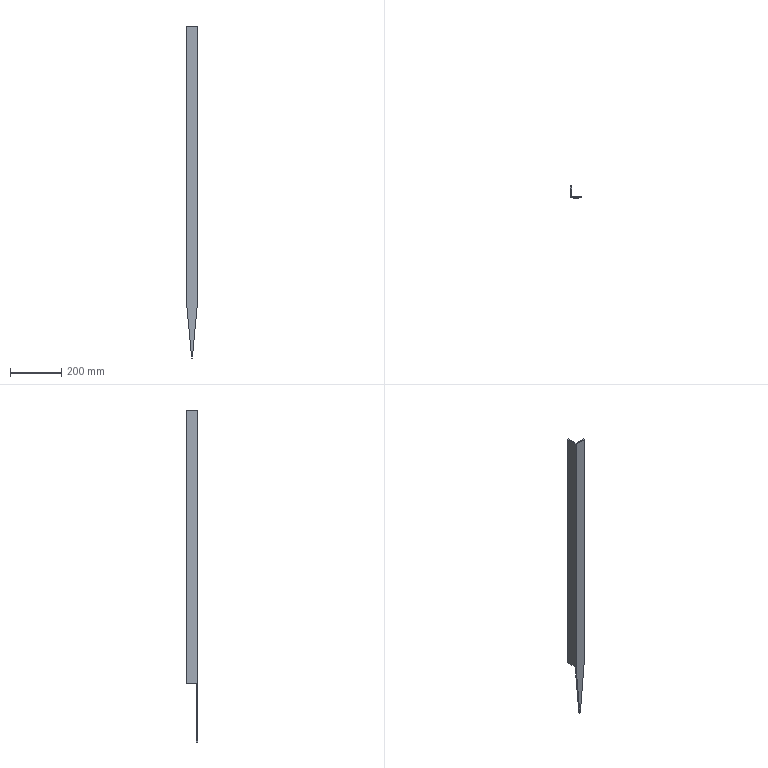Part | SolidWorks | features ICE 2, Extrusion 1 | 1 solid | 11 faces | box 45 x 45 x 1295 mm | volume 480925 mm3 | plane 11
STEP:
#1=CARTESIAN_POINT('',(-6.005,1.14,1295.4));
#2=VERTEX_POINT('',#1);
#3=CARTESIAN_POINT('',(-6.005,1.14,228.6));
#4=VERTEX_POINT('',#3);
#5=CARTESIAN_POINT('',(-6.005,1.14,1295.4));
#6=DIRECTION('',(0.,0.,-1.));
#7=VECTOR('',#6,1000.);
#8=LINE('',#5,#7);
#9=EDGE_CURVE('',#2,#4,#8,.T.);
#10=ORIENTED_EDGE('',*,*,#9,.T.);
#11=CARTESIAN_POINT('',(-11.005,1.14,228.6));
#12=VERTEX_POINT('',#11);
#13=CARTESIAN_POINT('',(-11.005,1.14,228.6));
#14=DIRECTION('',(1.,0.,0.));
#15=VECTOR('',#14,1000.);
#16=LINE('',#13,#15);
#17=EDGE_CURVE('',#12,#4,#16,.T.);
#18=ORIENTED_EDGE('',*,*,#17,.F.);
#19=CARTESIAN_POINT('',(-11.005,1.14,1295.4));
#20=VERTEX_POINT('',#19);
#21=CARTESIAN_POINT('',(-11.005,1.14,1295.4));
#22=DIRECTION('',(0.,0.,-1.));
#23=VECTOR('',#22,1000.);
#24=LINE('',#21,#23);
#25=EDGE_CURVE('',#20,#12,#24,.T.);
#26=ORIENTED_EDGE('',*,*,#25,.F.);
#27=CARTESIAN_POINT('',(-6.005,1.14,1295.4));
#28=DIRECTION('',(-1.,0.,0.));
#29=VECTOR('',#28,1000.);
#30=LINE('',#27,#29);
#31=EDGE_CURVE('',#2,#20,#30,.T.);
#32=ORIENTED_EDGE('',*,*,#31,.F.);
#33=EDGE_LOOP('',(#10,#18,#26,#32));
#34=FACE_OUTER_BOUND('',#33,.T.);
#35=CARTESIAN_POINT('',(-6.005,1.14,1295.4));
#36=DIRECTION('',(0.,-1.,0.));
#37=DIRECTION('',(0.,0.,-1.));
#38=AXIS2_PLACEMENT_3D('',#35,#36,#37);
#39=PLANE('',#38);
#40=ADVANCED_FACE('',(#34),#39,.F.);
#41=ORIENTED_EDGE('',*,*,#25,.T.);
#42=CARTESIAN_POINT('',(-11.005,-38.86,228.6));
#43=VERTEX_POINT('',#42);
#44=CARTESIAN_POINT('',(-11.005,1.14,228.6));
#45=DIRECTION('',(0.,-1.,0.));
#46=VECTOR('',#45,1000.);
#47=LINE('',#44,#46);
#48=EDGE_CURVE('',#12,#43,#47,.T.);
#49=ORIENTED_EDGE('',*,*,#48,.T.);
#50=CARTESIAN_POINT('',(-11.005,-43.86,228.6));
#51=VERTEX_POINT('',#50);
#52=CARTESIAN_POINT('',(-11.005,1.14,228.6));
#53=DIRECTION('',(0.,-1.,0.));
#54=VECTOR('',#53,1000.);
#55=LINE('',#52,#54);
#56=EDGE_CURVE('',#43,#51,#55,.T.);
#57=ORIENTED_EDGE('',*,*,#56,.T.);
#58=CARTESIAN_POINT('',(-11.005,-43.86,1295.4));
#59=VERTEX_POINT('',#58);
#60=CARTESIAN_POINT('',(-11.005,-43.86,1295.4));
#61=DIRECTION('',(0.,0.,-1.));
#62=VECTOR('',#61,1000.);
#63=LINE('',#60,#62);
#64=EDGE_CURVE('',#59,#51,#63,.T.);
#65=ORIENTED_EDGE('',*,*,#64,.F.);
#66=CARTESIAN_POINT('',(-11.005,1.14,1295.4));
#67=DIRECTION('',(0.,-1.,0.));
#68=VECTOR('',#67,1000.);
#69=LINE('',#66,#68);
#70=EDGE_CURVE('',#20,#59,#69,.T.);
#71=ORIENTED_EDGE('',*,*,#70,.F.);
#72=EDGE_LOOP('',(#41,#49,#57,#65,#71));
#73=FACE_OUTER_BOUND('',#72,.T.);
#74=CARTESIAN_POINT('',(-11.005,1.14,1295.4));
#75=DIRECTION('',(1.,0.,0.));
#76=DIRECTION('',(0.,1.,0.));
#77=AXIS2_PLACEMENT_3D('',#74,#75,#76);
#78=PLANE('',#77);
#79=ADVANCED_FACE('',(#73),#78,.F.);
#80=CARTESIAN_POINT('',(9.905,-43.86,0.));
#81=VERTEX_POINT('',#80);
#82=CARTESIAN_POINT('',(13.085,-43.86,0.));
#83=VERTEX_POINT('',#82);
#84=CARTESIAN_POINT('',(-11.005,-43.86,0.));
#85=DIRECTION('',(1.,0.,0.));
#86=VECTOR('',#85,1000.);
#87=LINE('',#84,#86);
#88=EDGE_CURVE('',#81,#83,#87,.T.);
#89=ORIENTED_EDGE('',*,*,#88,.T.);
#90=CARTESIAN_POINT('',(33.995,-43.86,228.6));
#91=VERTEX_POINT('',#90);
#92=CARTESIAN_POINT('',(33.995,-43.86,228.6));
#93=DIRECTION('',(-0.09109,0.,-0.9958));
#94=VECTOR('',#93,1000.);
#95=LINE('',#92,#94);
#96=EDGE_CURVE('',#91,#83,#95,.T.);
#97=ORIENTED_EDGE('',*,*,#96,.F.);
#98=CARTESIAN_POINT('',(33.995,-43.86,1295.4));
#99=VERTEX_POINT('',#98);
#100=CARTESIAN_POINT('',(33.995,-43.86,1295.4));
#101=DIRECTION('',(0.,0.,-1.));
#102=VECTOR('',#101,1000.);
#103=LINE('',#100,#102);
#104=EDGE_CURVE('',#99,#91,#103,.T.);
#105=ORIENTED_EDGE('',*,*,#104,.F.);
#106=CARTESIAN_POINT('',(-11.005,-43.86,1295.4));
#107=DIRECTION('',(1.,0.,0.));
#108=VECTOR('',#107,1000.);
#109=LINE('',#106,#108);
#110=EDGE_CURVE('',#59,#99,#109,.T.);
#111=ORIENTED_EDGE('',*,*,#110,.F.);
#112=ORIENTED_EDGE('',*,*,#64,.T.);
#113=CARTESIAN_POINT('',(-11.005,-43.86,228.6));
#114=DIRECTION('',(-0.09109,0.,0.9958));
#115=VECTOR('',#114,1000.);
#116=LINE('',#113,#115);
#117=EDGE_CURVE('',#81,#51,#116,.T.);
#118=ORIENTED_EDGE('',*,*,#117,.F.);
#119=EDGE_LOOP('',(#89,#97,#105,#111,#112,#118));
#120=FACE_OUTER_BOUND('',#119,.T.);
#121=CARTESIAN_POINT('',(-11.005,-43.86,1295.4));
#122=DIRECTION('',(0.,1.,0.));
#123=DIRECTION('',(0.,0.,1.));
#124=AXIS2_PLACEMENT_3D('',#121,#122,#123);
#125=PLANE('',#124);
#126=ADVANCED_FACE('',(#120),#125,.F.);
#127=ORIENTED_EDGE('',*,*,#104,.T.);
#128=CARTESIAN_POINT('',(33.995,-38.86,228.6));
#129=VERTEX_POINT('',#128);
#130=CARTESIAN_POINT('',(33.995,1.14,228.6));
#131=DIRECTION('',(0.,-1.,0.));
#132=VECTOR('',#131,1000.);
#133=LINE('',#130,#132);
#134=EDGE_CURVE('',#129,#91,#133,.T.);
#135=ORIENTED_EDGE('',*,*,#134,.F.);
#136=CARTESIAN_POINT('',(33.995,-38.86,1295.4));
#137=VERTEX_POINT('',#136);
#138=CARTESIAN_POINT('',(33.995,-38.86,1295.4));
#139=DIRECTION('',(0.,0.,-1.));
#140=VECTOR('',#139,1000.);
#141=LINE('',#138,#140);
#142=EDGE_CURVE('',#137,#129,#141,.T.);
#143=ORIENTED_EDGE('',*,*,#142,.F.);
#144=CARTESIAN_POINT('',(33.995,-43.86,1295.4));
#145=DIRECTION('',(0.,1.,0.));
#146=VECTOR('',#145,1000.);
#147=LINE('',#144,#146);
#148=EDGE_CURVE('',#99,#137,#147,.T.);
#149=ORIENTED_EDGE('',*,*,#148,.F.);
#150=EDGE_LOOP('',(#127,#135,#143,#149));
#151=FACE_OUTER_BOUND('',#150,.T.);
#152=CARTESIAN_POINT('',(33.995,-43.86,1295.4));
#153=DIRECTION('',(-1.,0.,0.));
#154=DIRECTION('',(0.,0.,1.));
#155=AXIS2_PLACEMENT_3D('',#152,#153,#154);
#156=PLANE('',#155);
#157=ADVANCED_FACE('',(#151),#156,.F.);
#158=ORIENTED_EDGE('',*,*,#142,.T.);
#159=CARTESIAN_POINT('',(13.085,-38.86,0.));
#160=VERTEX_POINT('',#159);
#161=CARTESIAN_POINT('',(130.765,-38.86,1286.548));
#162=DIRECTION('',(-0.09109,0.,-0.9958));
#163=VECTOR('',#162,1000.);
#164=LINE('',#161,#163);
#165=EDGE_CURVE('',#129,#160,#164,.T.);
#166=ORIENTED_EDGE('',*,*,#165,.T.);
#167=CARTESIAN_POINT('',(9.905,-38.86,0.));
#168=VERTEX_POINT('',#167);
#169=CARTESIAN_POINT('',(33.995,-38.86,0.));
#170=DIRECTION('',(-1.,0.,0.));
#171=VECTOR('',#170,1000.);
#172=LINE('',#169,#171);
#173=EDGE_CURVE('',#160,#168,#172,.T.);
#174=ORIENTED_EDGE('',*,*,#173,.T.);
#175=CARTESIAN_POINT('',(-107.402,-38.86,1282.466));
#176=DIRECTION('',(-0.09109,0.,0.9958));
#177=VECTOR('',#176,1000.);
#178=LINE('',#175,#177);
#179=EDGE_CURVE('',#168,#43,#178,.T.);
#180=ORIENTED_EDGE('',*,*,#179,.T.);
#181=CARTESIAN_POINT('',(-6.005,-38.86,228.6));
#182=VERTEX_POINT('',#181);
#183=CARTESIAN_POINT('',(-11.005,-38.86,228.6));
#184=DIRECTION('',(1.,0.,0.));
#185=VECTOR('',#184,1000.);
#186=LINE('',#183,#185);
#187=EDGE_CURVE('',#43,#182,#186,.T.);
#188=ORIENTED_EDGE('',*,*,#187,.T.);
#189=CARTESIAN_POINT('',(-6.005,-38.86,1295.4));
#190=VERTEX_POINT('',#189);
#191=CARTESIAN_POINT('',(-6.005,-38.86,1295.4));
#192=DIRECTION('',(0.,0.,-1.));
#193=VECTOR('',#192,1000.);
#194=LINE('',#191,#193);
#195=EDGE_CURVE('',#190,#182,#194,.T.);
#196=ORIENTED_EDGE('',*,*,#195,.F.);
#197=CARTESIAN_POINT('',(33.995,-38.86,1295.4));
#198=DIRECTION('',(-1.,0.,0.));
#199=VECTOR('',#198,1000.);
#200=LINE('',#197,#199);
#201=EDGE_CURVE('',#137,#190,#200,.T.);
#202=ORIENTED_EDGE('',*,*,#201,.F.);
#203=EDGE_LOOP('',(#158,#166,#174,#180,#188,#196,#202));
#204=FACE_OUTER_BOUND('',#203,.T.);
#205=CARTESIAN_POINT('',(33.995,-38.86,1295.4));
#206=DIRECTION('',(0.,-1.,0.));
#207=DIRECTION('',(1.,0.,0.));
#208=AXIS2_PLACEMENT_3D('',#205,#206,#207);
#209=PLANE('',#208);
#210=ADVANCED_FACE('',(#204),#209,.F.);
#211=ORIENTED_EDGE('',*,*,#195,.T.);
#212=CARTESIAN_POINT('',(-6.005,1.14,228.6));
#213=DIRECTION('',(0.,-1.,0.));
#214=VECTOR('',#213,1000.);
#215=LINE('',#212,#214);
#216=EDGE_CURVE('',#4,#182,#215,.T.);
#217=ORIENTED_EDGE('',*,*,#216,.F.);
#218=ORIENTED_EDGE('',*,*,#9,.F.);
#219=CARTESIAN_POINT('',(-6.005,-38.86,1295.4));
#220=DIRECTION('',(0.,1.,0.));
#221=VECTOR('',#220,1000.);
#222=LINE('',#219,#221);
#223=EDGE_CURVE('',#190,#2,#222,.T.);
#224=ORIENTED_EDGE('',*,*,#223,.F.);
#225=EDGE_LOOP('',(#211,#217,#218,#224));
#226=FACE_OUTER_BOUND('',#225,.T.);
#227=CARTESIAN_POINT('',(-6.005,-38.86,1295.4));
#228=DIRECTION('',(-1.,0.,0.));
#229=DIRECTION('',(0.,-1.,0.));
#230=AXIS2_PLACEMENT_3D('',#227,#228,#229);
#231=PLANE('',#230);
#232=ADVANCED_FACE('',(#226),#231,.F.);
#233=ORIENTED_EDGE('',*,*,#31,.T.);
#234=ORIENTED_EDGE('',*,*,#70,.T.);
#235=ORIENTED_EDGE('',*,*,#110,.T.);
#236=ORIENTED_EDGE('',*,*,#148,.T.);
#237=ORIENTED_EDGE('',*,*,#201,.T.);
#238=ORIENTED_EDGE('',*,*,#223,.T.);
#239=EDGE_LOOP('',(#233,#234,#235,#236,#237,#238));
#240=FACE_OUTER_BOUND('',#239,.T.);
#241=CARTESIAN_POINT('',(-11.005,1.14,1295.4));
#242=DIRECTION('',(0.,0.,1.));
#243=DIRECTION('',(1.,0.,0.));
#244=AXIS2_PLACEMENT_3D('',#241,#242,#243);
#245=PLANE('',#244);
#246=ADVANCED_FACE('',(#240),#245,.T.);
#247=ORIENTED_EDGE('',*,*,#173,.F.);
#248=CARTESIAN_POINT('',(13.085,1.14,0.));
#249=DIRECTION('',(0.,-1.,0.));
#250=VECTOR('',#249,1000.);
#251=LINE('',#248,#250);
#252=EDGE_CURVE('',#160,#83,#251,.T.);
#253=ORIENTED_EDGE('',*,*,#252,.T.);
#254=ORIENTED_EDGE('',*,*,#88,.F.);
#255=CARTESIAN_POINT('',(9.905,1.14,0.));
#256=DIRECTION('',(0.,1.,0.));
#257=VECTOR('',#256,1000.);
#258=LINE('',#255,#257);
#259=EDGE_CURVE('',#81,#168,#258,.T.);
#260=ORIENTED_EDGE('',*,*,#259,.T.);
#261=EDGE_LOOP('',(#247,#253,#254,#260));
#262=FACE_OUTER_BOUND('',#261,.T.);
#263=CARTESIAN_POINT('',(-11.005,1.14,0.));
#264=DIRECTION('',(0.,0.,1.));
#265=DIRECTION('',(1.,0.,0.));
#266=AXIS2_PLACEMENT_3D('',#263,#264,#265);
#267=PLANE('',#266);
#268=ADVANCED_FACE('',(#262),#267,.F.);
#269=ORIENTED_EDGE('',*,*,#56,.F.);
#270=ORIENTED_EDGE('',*,*,#179,.F.);
#271=ORIENTED_EDGE('',*,*,#259,.F.);
#272=ORIENTED_EDGE('',*,*,#117,.T.);
#273=EDGE_LOOP('',(#269,#270,#271,#272));
#274=FACE_OUTER_BOUND('',#273,.T.);
#275=CARTESIAN_POINT('',(-11.005,1.14,228.6));
#276=DIRECTION('',(0.9958,0.,0.09109));
#277=DIRECTION('',(0.09109,0.,-0.9958));
#278=AXIS2_PLACEMENT_3D('',#275,#276,#277);
#279=PLANE('',#278);
#280=ADVANCED_FACE('',(#274),#279,.F.);
#281=ORIENTED_EDGE('',*,*,#134,.T.);
#282=ORIENTED_EDGE('',*,*,#96,.T.);
#283=ORIENTED_EDGE('',*,*,#252,.F.);
#284=ORIENTED_EDGE('',*,*,#165,.F.);
#285=EDGE_LOOP('',(#281,#282,#283,#284));
#286=FACE_OUTER_BOUND('',#285,.T.);
#287=CARTESIAN_POINT('',(33.995,1.14,228.6));
#288=DIRECTION('',(-0.9958,0.,0.09109));
#289=DIRECTION('',(0.09109,0.,0.9958));
#290=AXIS2_PLACEMENT_3D('',#287,#288,#289);
#291=PLANE('',#290);
#292=ADVANCED_FACE('',(#286),#291,.F.);
#293=ORIENTED_EDGE('',*,*,#216,.T.);
#294=ORIENTED_EDGE('',*,*,#187,.F.);
#295=ORIENTED_EDGE('',*,*,#48,.F.);
#296=ORIENTED_EDGE('',*,*,#17,.T.);
#297=EDGE_LOOP('',(#293,#294,#295,#296));
#298=FACE_OUTER_BOUND('',#297,.T.);
#299=CARTESIAN_POINT('',(-11.005,1.14,228.6));
#300=DIRECTION('',(0.,0.,1.));
#301=DIRECTION('',(0.,-1.,0.));
#302=AXIS2_PLACEMENT_3D('',#299,#300,#301);
#303=PLANE('',#302);
#304=ADVANCED_FACE('',(#298),#303,.F.);
#305=CLOSED_SHELL('',(#40,#79,#126,#157,#210,#232,#246,#268,#280,#292,#304));
#306=MANIFOLD_SOLID_BREP('',#305);
#307=CARTESIAN_POINT('',(0.,0.,0.));
#308=DIRECTION('',(0.,0.,1.));
#309=DIRECTION('',(1.,0.,0.));
#310=AXIS2_PLACEMENT_3D('',#307,#308,#309);
#311=(LENGTH_UNIT()NAMED_UNIT(*)SI_UNIT(.MILLI.,.METRE.));
#312=UNCERTAINTY_MEASURE_WITH_UNIT(LENGTH_MEASURE(0.00001),#311,'','');
#313=(NAMED_UNIT(*)PLANE_ANGLE_UNIT()SI_UNIT($,.RADIAN.));
#314=(NAMED_UNIT(*)SI_UNIT($,.STERADIAN.)SOLID_ANGLE_UNIT());
#315=(GEOMETRIC_REPRESENTATION_CONTEXT(3)GLOBAL_UNCERTAINTY_ASSIGNED_CONTEXT((#312))GLOBAL_UNIT_ASSIGNED_CONTEXT((#311,#313,#314))REPRESENTATION_CONTEXT('',''));
#316=ADVANCED_BREP_SHAPE_REPRESENTATION('',(#306,#310),#315);